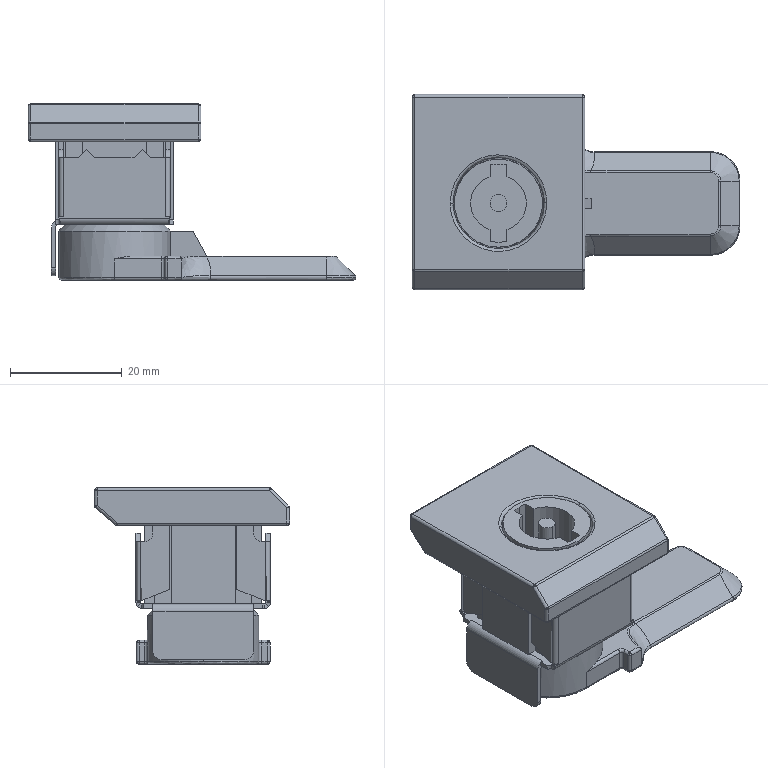Part | STEP file | Cylinder lock MS813-Shengjiu | 4 solids | 391 faces | box 58.793 x 35 x 31.6 mm | volume 16415 mm3 | plane 176 | cylinder 124 | spline 77 | cone 14 | commonest cylinder face diameters 1 x52 3 x14 2 x13 1.5 x8 10 x6 12 x5